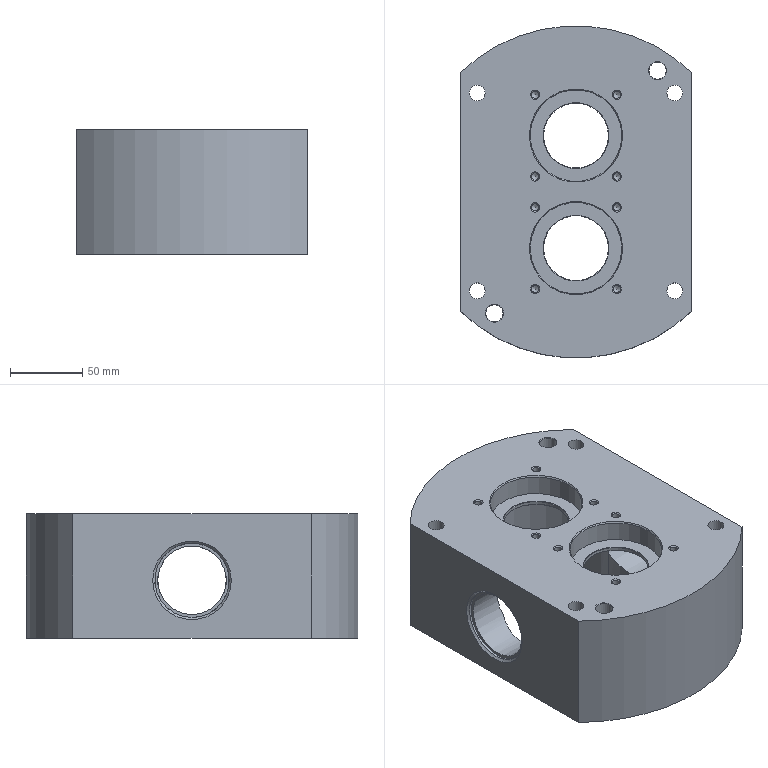Part | 1 solid | 97 faces | box 160 x 230 x 86 mm | volume 1383228 mm3 | cone 44 | cylinder 40 | plane 13 | commonest cylinder face diameters 5 x8 6.8 x6 110.4 x6 11 x4 17 x4 12 x2